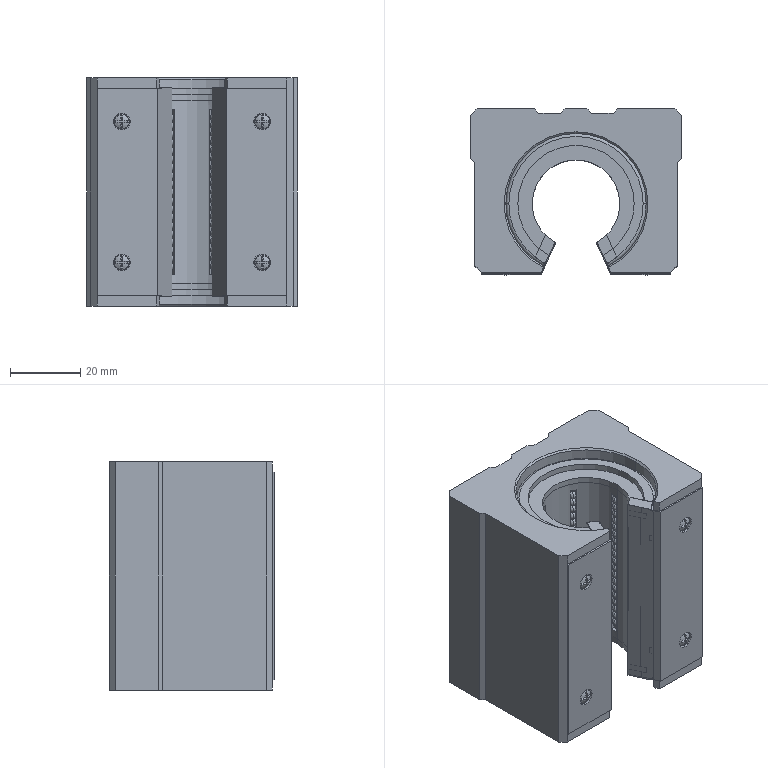Part | SolidWorks | features BaseBody 5 | 5 solids | 734 faces | box 60 x 47.265 x 65 mm | volume 129093 mm3 | plane 399 | sphere 232 | cylinder 75 | torus 14 | cone 14 | commonest cylinder face diameters 36.25 x12 40 x12 25 x9 4.32 x8 4.8 x8 6 x8